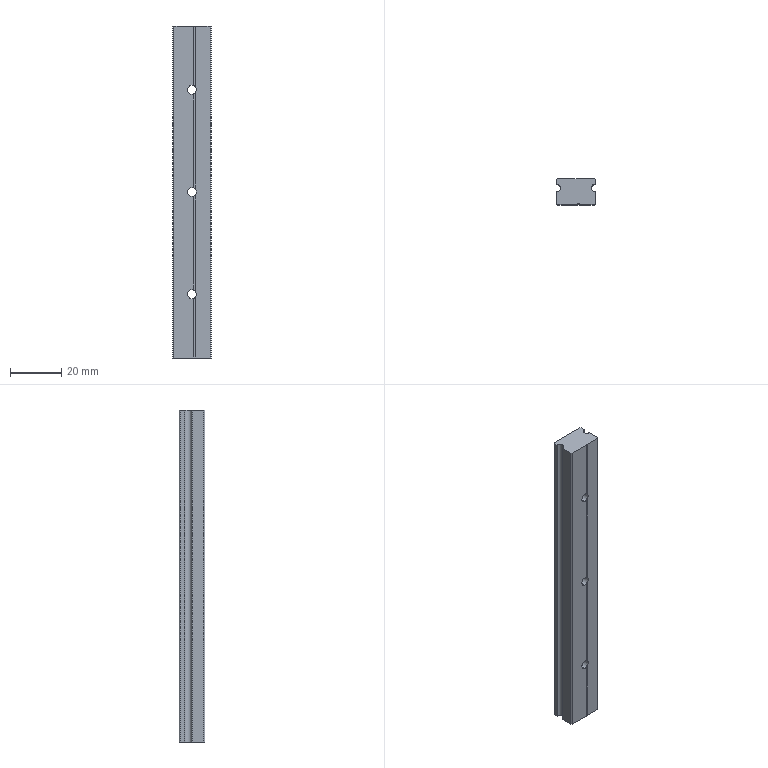Part | STEP file | MGN15H-130-01-cc | 1 solid | 35 faces | box 15 x 10 x 130 mm | volume 18038 mm3 | cylinder 19 | plane 16 | commonest cylinder face diameters 3.5 x6 6 x6 0.6 x4 3 x3